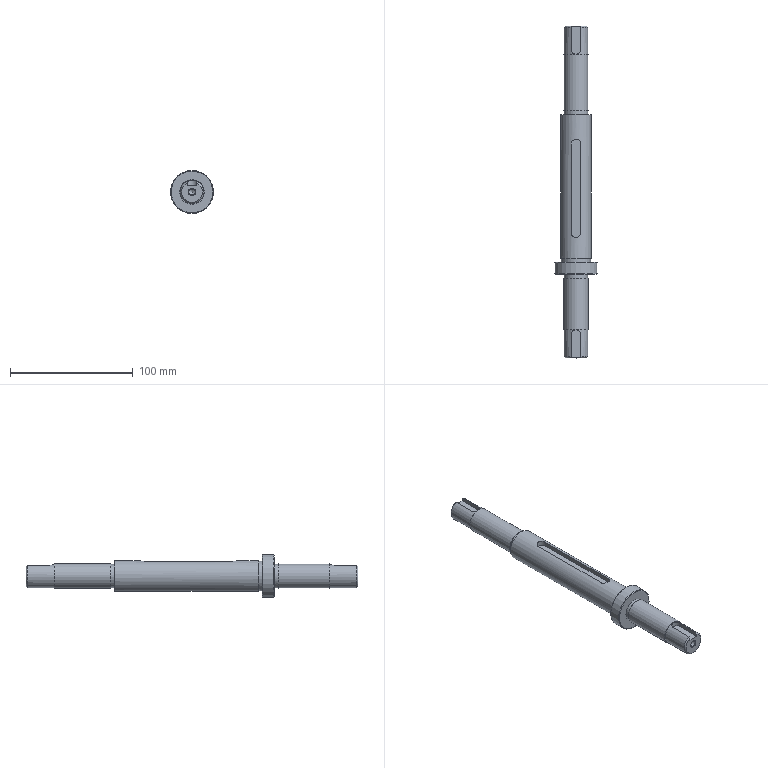Part | STEP file | 冲床-300配套压波_id562_x_t | 1 solid | 49 faces | box 35 x 270 x 35 mm | volume 104906 mm3 | plane 21 | cylinder 17 | cone 11 | commonest cylinder face diameters 19 x4 5 x2 6.8 x2 8 x2 8.04 x2 20 x2
STEP:
#1=CARTESIAN_POINT('',(1267.,-67.,104.));
#2=VERTEX_POINT('',#1);
#3=CARTESIAN_POINT('',(1250.,-67.,104.));
#4=DIRECTION('',(0.,-1.,0.));
#5=DIRECTION('',(1.,0.,0.));
#6=AXIS2_PLACEMENT_3D('',#3,#4,#5);
#7=CIRCLE('',#6,17.);
#8=EDGE_CURVE('',#2,#2,#7,.T.);
#9=ORIENTED_EDGE('',*,*,#8,.T.);
#10=EDGE_LOOP('',(#9));
#11=FACE_BOUND('',#10,.T.);
#12=CARTESIAN_POINT('',(1259.5,-67.,104.));
#13=VERTEX_POINT('',#12);
#14=CARTESIAN_POINT('',(1250.,-67.,104.));
#15=DIRECTION('',(0.,-1.,0.));
#16=DIRECTION('',(1.,0.,0.));
#17=AXIS2_PLACEMENT_3D('',#14,#15,#16);
#18=CIRCLE('',#17,9.5);
#19=EDGE_CURVE('',#13,#13,#18,.T.);
#20=ORIENTED_EDGE('',*,*,#19,.F.);
#21=EDGE_LOOP('',(#20));
#22=FACE_BOUND('',#21,.T.);
#23=CARTESIAN_POINT('',(1250.,-67.,104.));
#24=DIRECTION('',(0.,-1.,0.));
#25=DIRECTION('',(1.,0.,0.));
#26=AXIS2_PLACEMENT_3D('',#23,#24,#25);
#27=PLANE('',#26);
#28=ADVANCED_FACE('',(#11,#22),#27,.T.);
#29=CARTESIAN_POINT('',(1233.,-57.,104.));
#30=VERTEX_POINT('',#29);
#31=CARTESIAN_POINT('',(1250.,-57.,104.));
#32=DIRECTION('',(0.,1.,0.));
#33=DIRECTION('',(-1.,0.,0.));
#34=AXIS2_PLACEMENT_3D('',#31,#32,#33);
#35=CIRCLE('',#34,17.);
#36=EDGE_CURVE('',#30,#30,#35,.T.);
#37=ORIENTED_EDGE('',*,*,#36,.T.);
#38=EDGE_LOOP('',(#37));
#39=FACE_BOUND('',#38,.T.);
#40=CARTESIAN_POINT('',(1238.,-57.,104.));
#41=VERTEX_POINT('',#40);
#42=CARTESIAN_POINT('',(1250.,-57.,104.));
#43=DIRECTION('',(0.,1.,0.));
#44=DIRECTION('',(-1.,0.,0.));
#45=AXIS2_PLACEMENT_3D('',#42,#43,#44);
#46=CIRCLE('',#45,12.);
#47=EDGE_CURVE('',#41,#41,#46,.T.);
#48=ORIENTED_EDGE('',*,*,#47,.F.);
#49=EDGE_LOOP('',(#48));
#50=FACE_BOUND('',#49,.T.);
#51=CARTESIAN_POINT('',(1250.,-57.,104.));
#52=DIRECTION('',(0.,1.,0.));
#53=DIRECTION('',(-1.,0.,0.));
#54=AXIS2_PLACEMENT_3D('',#51,#52,#53);
#55=PLANE('',#54);
#56=ADVANCED_FACE('',(#39,#50),#55,.T.);
#57=CARTESIAN_POINT('',(1250.,-66.5,121.5));
#58=VERTEX_POINT('',#57);
#59=CARTESIAN_POINT('',(1250.,-66.5,104.));
#60=DIRECTION('',(0.,1.,0.));
#61=DIRECTION('',(0.,0.,1.));
#62=AXIS2_PLACEMENT_3D('',#59,#60,#61);
#63=CIRCLE('',#62,17.5);
#64=EDGE_CURVE('',#58,#58,#63,.T.);
#65=ORIENTED_EDGE('',*,*,#64,.T.);
#66=EDGE_LOOP('',(#65));
#67=FACE_BOUND('',#66,.T.);
#68=CARTESIAN_POINT('',(1250.,-57.5,86.5));
#69=VERTEX_POINT('',#68);
#70=CARTESIAN_POINT('',(1250.,-57.5,104.));
#71=DIRECTION('',(0.,-1.,0.));
#72=DIRECTION('',(0.,0.,-1.));
#73=AXIS2_PLACEMENT_3D('',#70,#71,#72);
#74=CIRCLE('',#73,17.5);
#75=EDGE_CURVE('',#69,#69,#74,.T.);
#76=ORIENTED_EDGE('',*,*,#75,.T.);
#77=EDGE_LOOP('',(#76));
#78=FACE_BOUND('',#77,.T.);
#79=CARTESIAN_POINT('',(1250.,-54.,104.));
#80=DIRECTION('',(0.,-1.,0.));
#81=DIRECTION('',(1.,0.,0.));
#82=AXIS2_PLACEMENT_3D('',#79,#80,#81);
#83=CYLINDRICAL_SURFACE('',#82,17.5);
#84=ADVANCED_FACE('',(#67,#78),#83,.T.);
#85=ORIENTED_EDGE('',*,*,#8,.F.);
#86=EDGE_LOOP('',(#85));
#87=FACE_BOUND('',#86,.T.);
#88=ORIENTED_EDGE('',*,*,#64,.F.);
#89=EDGE_LOOP('',(#88));
#90=FACE_BOUND('',#89,.T.);
#91=CARTESIAN_POINT('',(1250.,-66.5,104.));
#92=DIRECTION('',(0.,1.,0.));
#93=DIRECTION('',(0.,0.,1.));
#94=AXIS2_PLACEMENT_3D('',#91,#92,#93);
#95=CONICAL_SURFACE('',#94,17.5,45.);
#96=ADVANCED_FACE('',(#87,#90),#95,.T.);
#97=ORIENTED_EDGE('',*,*,#36,.F.);
#98=EDGE_LOOP('',(#97));
#99=FACE_BOUND('',#98,.T.);
#100=ORIENTED_EDGE('',*,*,#75,.F.);
#101=EDGE_LOOP('',(#100));
#102=FACE_BOUND('',#101,.T.);
#103=CARTESIAN_POINT('',(1250.,-57.5,104.));
#104=DIRECTION('',(0.,-1.,0.));
#105=DIRECTION('',(0.,0.,-1.));
#106=AXIS2_PLACEMENT_3D('',#103,#104,#105);
#107=CONICAL_SURFACE('',#106,17.5,45.);
#108=ADVANCED_FACE('',(#99,#102),#107,.T.);
#109=CARTESIAN_POINT('',(1250.,-54.,92.));
#110=VERTEX_POINT('',#109);
#111=CARTESIAN_POINT('',(1250.,-54.,104.));
#112=DIRECTION('',(0.,-1.,0.));
#113=DIRECTION('',(0.,0.,-1.));
#114=AXIS2_PLACEMENT_3D('',#111,#112,#113);
#115=CIRCLE('',#114,12.);
#116=EDGE_CURVE('',#110,#110,#115,.T.);
#117=ORIENTED_EDGE('',*,*,#116,.F.);
#118=EDGE_LOOP('',(#117));
#119=FACE_BOUND('',#118,.T.);
#120=CARTESIAN_POINT('',(1237.5,-54.,104.));
#121=VERTEX_POINT('',#120);
#122=CARTESIAN_POINT('',(1250.,-54.,104.));
#123=DIRECTION('',(0.,1.,0.));
#124=DIRECTION('',(-1.,0.,0.));
#125=AXIS2_PLACEMENT_3D('',#122,#123,#124);
#126=CIRCLE('',#125,12.5);
#127=EDGE_CURVE('',#121,#121,#126,.T.);
#128=ORIENTED_EDGE('',*,*,#127,.F.);
#129=EDGE_LOOP('',(#128));
#130=FACE_BOUND('',#129,.T.);
#131=CARTESIAN_POINT('',(1250.,-54.,104.));
#132=DIRECTION('',(0.,-1.,0.));
#133=DIRECTION('',(0.,0.,-1.));
#134=AXIS2_PLACEMENT_3D('',#131,#132,#133);
#135=PLANE('',#134);
#136=ADVANCED_FACE('',(#119,#130),#135,.T.);
#137=ORIENTED_EDGE('',*,*,#47,.T.);
#138=EDGE_LOOP('',(#137));
#139=FACE_BOUND('',#138,.T.);
#140=ORIENTED_EDGE('',*,*,#116,.T.);
#141=EDGE_LOOP('',(#140));
#142=FACE_BOUND('',#141,.T.);
#143=CARTESIAN_POINT('',(1250.,-57.,104.));
#144=DIRECTION('',(0.,1.,0.));
#145=DIRECTION('',(0.,0.,1.));
#146=AXIS2_PLACEMENT_3D('',#143,#144,#145);
#147=CYLINDRICAL_SURFACE('',#146,12.);
#148=ADVANCED_FACE('',(#139,#142),#147,.T.);
#149=CARTESIAN_POINT('',(1250.,66.,114.));
#150=VERTEX_POINT('',#149);
#151=CARTESIAN_POINT('',(1250.,66.,104.));
#152=DIRECTION('',(0.,-1.,0.));
#153=DIRECTION('',(0.,0.,1.));
#154=AXIS2_PLACEMENT_3D('',#151,#152,#153);
#155=CIRCLE('',#154,10.);
#156=EDGE_CURVE('',#150,#150,#155,.T.);
#157=ORIENTED_EDGE('',*,*,#156,.F.);
#158=EDGE_LOOP('',(#157));
#159=FACE_BOUND('',#158,.T.);
#160=CARTESIAN_POINT('',(1250.,112.,114.));
#161=VERTEX_POINT('',#160);
#162=CARTESIAN_POINT('',(1250.,112.,104.));
#163=DIRECTION('',(0.,-1.,0.));
#164=DIRECTION('',(0.,0.,1.));
#165=AXIS2_PLACEMENT_3D('',#162,#163,#164);
#166=CIRCLE('',#165,10.);
#167=EDGE_CURVE('',#161,#161,#166,.T.);
#168=ORIENTED_EDGE('',*,*,#167,.T.);
#169=EDGE_LOOP('',(#168));
#170=FACE_BOUND('',#169,.T.);
#171=CARTESIAN_POINT('',(1250.,92.,104.));
#172=DIRECTION('',(0.,1.,0.));
#173=DIRECTION('',(1.,0.,0.));
#174=AXIS2_PLACEMENT_3D('',#171,#172,#173);
#175=CYLINDRICAL_SURFACE('',#174,10.);
#176=ADVANCED_FACE('',(#159,#170),#175,.T.);
#177=ORIENTED_EDGE('',*,*,#156,.T.);
#178=EDGE_LOOP('',(#177));
#179=FACE_BOUND('',#178,.T.);
#180=CARTESIAN_POINT('',(1250.,66.,113.5));
#181=VERTEX_POINT('',#180);
#182=CARTESIAN_POINT('',(1250.,66.,104.));
#183=DIRECTION('',(0.,-1.,0.));
#184=DIRECTION('',(0.,0.,1.));
#185=AXIS2_PLACEMENT_3D('',#182,#183,#184);
#186=CIRCLE('',#185,9.5);
#187=EDGE_CURVE('',#181,#181,#186,.T.);
#188=ORIENTED_EDGE('',*,*,#187,.F.);
#189=EDGE_LOOP('',(#188));
#190=FACE_BOUND('',#189,.T.);
#191=CARTESIAN_POINT('',(1250.,66.,104.));
#192=DIRECTION('',(0.,1.,0.));
#193=DIRECTION('',(0.,0.,1.));
#194=AXIS2_PLACEMENT_3D('',#191,#192,#193);
#195=PLANE('',#194);
#196=ADVANCED_FACE('',(#179,#190),#195,.F.);
#197=CARTESIAN_POINT('',(1250.,63.,94.5));
#198=VERTEX_POINT('',#197);
#199=CARTESIAN_POINT('',(1250.,63.,104.));
#200=DIRECTION('',(0.,1.,0.));
#201=DIRECTION('',(0.,0.,-1.));
#202=AXIS2_PLACEMENT_3D('',#199,#200,#201);
#203=CIRCLE('',#202,9.5);
#204=EDGE_CURVE('',#198,#198,#203,.T.);
#205=ORIENTED_EDGE('',*,*,#204,.T.);
#206=EDGE_LOOP('',(#205));
#207=FACE_BOUND('',#206,.T.);
#208=ORIENTED_EDGE('',*,*,#187,.T.);
#209=EDGE_LOOP('',(#208));
#210=FACE_BOUND('',#209,.T.);
#211=CARTESIAN_POINT('',(1250.,92.,104.));
#212=DIRECTION('',(0.,1.,0.));
#213=DIRECTION('',(0.,0.,1.));
#214=AXIS2_PLACEMENT_3D('',#211,#212,#213);
#215=CYLINDRICAL_SURFACE('',#214,9.5);
#216=ADVANCED_FACE('',(#207,#210),#215,.T.);
#217=CARTESIAN_POINT('',(1254.02,38.98,112.3));
#218=VERTEX_POINT('',#217);
#219=CARTESIAN_POINT('',(1245.98,38.98,112.3));
#220=VERTEX_POINT('',#219);
#221=CARTESIAN_POINT('',(1250.,38.98,112.3));
#222=DIRECTION('',(0.,0.,1.));
#223=DIRECTION('',(1.,0.,0.));
#224=AXIS2_PLACEMENT_3D('',#221,#222,#223);
#225=CIRCLE('',#224,4.02);
#226=EDGE_CURVE('',#218,#220,#225,.T.);
#227=ORIENTED_EDGE('',*,*,#226,.T.);
#228=CARTESIAN_POINT('',(1245.98,-32.98,112.3));
#229=VERTEX_POINT('',#228);
#230=CARTESIAN_POINT('',(1245.98,43.,112.3));
#231=DIRECTION('',(0.,1.,0.));
#232=VECTOR('',#231,1.);
#233=LINE('',#230,#232);
#234=EDGE_CURVE('',#229,#220,#233,.T.);
#235=ORIENTED_EDGE('',*,*,#234,.F.);
#236=CARTESIAN_POINT('',(1254.02,-32.98,112.3));
#237=VERTEX_POINT('',#236);
#238=CARTESIAN_POINT('',(1250.,-32.98,112.3));
#239=DIRECTION('',(0.,0.,1.));
#240=DIRECTION('',(1.,0.,0.));
#241=AXIS2_PLACEMENT_3D('',#238,#239,#240);
#242=CIRCLE('',#241,4.02);
#243=EDGE_CURVE('',#229,#237,#242,.T.);
#244=ORIENTED_EDGE('',*,*,#243,.T.);
#245=CARTESIAN_POINT('',(1254.02,43.,112.3));
#246=DIRECTION('',(0.,1.,0.));
#247=VECTOR('',#246,1.);
#248=LINE('',#245,#247);
#249=EDGE_CURVE('',#237,#218,#248,.T.);
#250=ORIENTED_EDGE('',*,*,#249,.T.);
#251=EDGE_LOOP('',(#227,#235,#244,#250));
#252=FACE_OUTER_BOUND('',#251,.T.);
#253=CARTESIAN_POINT('',(1254.02,43.,112.3));
#254=DIRECTION('',(0.,0.,1.));
#255=DIRECTION('',(1.,0.,0.));
#256=AXIS2_PLACEMENT_3D('',#253,#254,#255);
#257=PLANE('',#256);
#258=ADVANCED_FACE('',(#252),#257,.T.);
#259=CARTESIAN_POINT('',(1250.,63.,91.5));
#260=VERTEX_POINT('',#259);
#261=CARTESIAN_POINT('',(1250.,63.,104.));
#262=DIRECTION('',(0.,1.,0.));
#263=DIRECTION('',(0.,0.,-1.));
#264=AXIS2_PLACEMENT_3D('',#261,#262,#263);
#265=CIRCLE('',#264,12.5);
#266=EDGE_CURVE('',#260,#260,#265,.T.);
#267=ORIENTED_EDGE('',*,*,#266,.T.);
#268=EDGE_LOOP('',(#267));
#269=FACE_BOUND('',#268,.T.);
#270=ORIENTED_EDGE('',*,*,#204,.F.);
#271=EDGE_LOOP('',(#270));
#272=FACE_BOUND('',#271,.T.);
#273=CARTESIAN_POINT('',(1250.,63.,104.));
#274=DIRECTION('',(0.,-1.,0.));
#275=DIRECTION('',(0.,0.,1.));
#276=AXIS2_PLACEMENT_3D('',#273,#274,#275);
#277=PLANE('',#276);
#278=ADVANCED_FACE('',(#269,#272),#277,.F.);
#279=CARTESIAN_POINT('',(1254.02,-32.98,115.836));
#280=VERTEX_POINT('',#279);
#281=CARTESIAN_POINT('',(1254.02,-32.98,116.5));
#282=DIRECTION('',(0.,0.,1.));
#283=VECTOR('',#282,1.);
#284=LINE('',#281,#283);
#285=EDGE_CURVE('',#237,#280,#284,.T.);
#286=ORIENTED_EDGE('',*,*,#285,.F.);
#287=ORIENTED_EDGE('',*,*,#243,.F.);
#288=CARTESIAN_POINT('',(1245.98,-32.98,115.836));
#289=VERTEX_POINT('',#288);
#290=CARTESIAN_POINT('',(1245.98,-32.98,112.4));
#291=DIRECTION('',(0.,0.,-1.));
#292=VECTOR('',#291,1.);
#293=LINE('',#290,#292);
#294=EDGE_CURVE('',#289,#229,#293,.T.);
#295=ORIENTED_EDGE('',*,*,#294,.F.);
#296=CARTESIAN_POINT('',(1254.02,-32.98,115.836));
#297=CARTESIAN_POINT('',(1254.02,-33.417,115.836));
#298=CARTESIAN_POINT('',(1253.947,-33.86,115.862));
#299=CARTESIAN_POINT('',(1253.807,-34.271,115.906));
#300=CARTESIAN_POINT('',(1253.668,-34.682,115.951));
#301=CARTESIAN_POINT('',(1253.459,-35.073,116.015));
#302=CARTESIAN_POINT('',(1253.198,-35.416,116.084));
#303=CARTESIAN_POINT('',(1252.928,-35.77,116.155));
#304=CARTESIAN_POINT('',(1252.596,-36.082,116.233));
#305=CARTESIAN_POINT('',(1252.224,-36.328,116.3));
#306=CARTESIAN_POINT('',(1251.844,-36.581,116.369));
#307=CARTESIAN_POINT('',(1251.413,-36.772,116.428));
#308=CARTESIAN_POINT('',(1250.966,-36.882,116.463));
#309=CARTESIAN_POINT('',(1250.535,-36.989,116.496));
#310=CARTESIAN_POINT('',(1250.076,-37.024,116.508));
#311=CARTESIAN_POINT('',(1249.632,-36.983,116.495));
#312=CARTESIAN_POINT('',(1249.204,-36.944,116.482));
#313=CARTESIAN_POINT('',(1248.778,-36.833,116.446));
#314=CARTESIAN_POINT('',(1248.387,-36.662,116.395));
#315=CARTESIAN_POINT('',(1247.99,-36.488,116.344));
#316=CARTESIAN_POINT('',(1247.62,-36.248,116.276));
#317=CARTESIAN_POINT('',(1247.301,-35.959,116.205));
#318=CARTESIAN_POINT('',(1246.969,-35.658,116.132));
#319=CARTESIAN_POINT('',(1246.683,-35.296,116.054));
#320=CARTESIAN_POINT('',(1246.468,-34.9,115.991));
#321=CARTESIAN_POINT('',(1246.251,-34.5,115.927));
#322=CARTESIAN_POINT('',(1246.099,-34.053,115.876));
#323=CARTESIAN_POINT('',(1246.028,-33.599,115.852));
#324=CARTESIAN_POINT('',(1245.996,-33.395,115.841));
#325=CARTESIAN_POINT('',(1245.98,-33.187,115.836));
#326=CARTESIAN_POINT('',(1245.98,-32.98,115.836));
#327=B_SPLINE_CURVE_WITH_KNOTS('',3,(#296,#297,#298,#299,#300,#301,#302,#303,#304,#305,#306,#307,#308,#309,#310,#311,#312,#313,#314,#315,#316,#317,#318,#319,#320,#321,#322,#323,#324,#325,#326),.UNSPECIFIED.,.F.,.F.,(4,3,3,3,3,3,3,3,3,3,4),(0.,0.1036,0.207,0.3138,0.4233,0.5292,0.6311,0.7343,0.8422,0.9514,1.),.UNSPECIFIED.);
#328=EDGE_CURVE('',#280,#289,#327,.T.);
#329=ORIENTED_EDGE('',*,*,#328,.F.);
#330=EDGE_LOOP('',(#286,#287,#295,#329));
#331=FACE_OUTER_BOUND('',#330,.T.);
#332=CARTESIAN_POINT('',(1250.,-32.98,116.5));
#333=DIRECTION('',(0.,0.,-1.));
#334=DIRECTION('',(-1.,0.,0.));
#335=AXIS2_PLACEMENT_3D('',#332,#333,#334);
#336=CYLINDRICAL_SURFACE('',#335,4.02);
#337=ADVANCED_FACE('',(#331),#336,.F.);
#338=CARTESIAN_POINT('',(1254.02,38.98,115.836));
#339=VERTEX_POINT('',#338);
#340=CARTESIAN_POINT('',(1254.02,173.,115.836));
#341=DIRECTION('',(0.,1.,0.));
#342=VECTOR('',#341,1.);
#343=LINE('',#340,#342);
#344=EDGE_CURVE('',#280,#339,#343,.T.);
#345=ORIENTED_EDGE('',*,*,#344,.T.);
#346=CARTESIAN_POINT('',(1254.02,38.98,116.5));
#347=DIRECTION('',(0.,0.,-1.));
#348=VECTOR('',#347,1.);
#349=LINE('',#346,#348);
#350=EDGE_CURVE('',#339,#218,#349,.T.);
#351=ORIENTED_EDGE('',*,*,#350,.T.);
#352=ORIENTED_EDGE('',*,*,#249,.F.);
#353=ORIENTED_EDGE('',*,*,#285,.T.);
#354=EDGE_LOOP('',(#345,#351,#352,#353));
#355=FACE_OUTER_BOUND('',#354,.T.);
#356=CARTESIAN_POINT('',(1254.02,43.,116.5));
#357=DIRECTION('',(-1.,0.,0.));
#358=DIRECTION('',(0.,0.,1.));
#359=AXIS2_PLACEMENT_3D('',#356,#357,#358);
#360=PLANE('',#359);
#361=ADVANCED_FACE('',(#355),#360,.T.);
#362=CARTESIAN_POINT('',(1245.98,38.98,115.836));
#363=VERTEX_POINT('',#362);
#364=CARTESIAN_POINT('',(1245.98,38.98,112.4));
#365=DIRECTION('',(0.,0.,1.));
#366=VECTOR('',#365,1.);
#367=LINE('',#364,#366);
#368=EDGE_CURVE('',#220,#363,#367,.T.);
#369=ORIENTED_EDGE('',*,*,#368,.F.);
#370=ORIENTED_EDGE('',*,*,#226,.F.);
#371=ORIENTED_EDGE('',*,*,#350,.F.);
#372=CARTESIAN_POINT('',(1245.98,38.98,115.836));
#373=CARTESIAN_POINT('',(1245.98,39.417,115.836));
#374=CARTESIAN_POINT('',(1246.053,39.86,115.862));
#375=CARTESIAN_POINT('',(1246.193,40.271,115.906));
#376=CARTESIAN_POINT('',(1246.332,40.682,115.951));
#377=CARTESIAN_POINT('',(1246.541,41.073,116.015));
#378=CARTESIAN_POINT('',(1246.802,41.416,116.084));
#379=CARTESIAN_POINT('',(1247.072,41.77,116.155));
#380=CARTESIAN_POINT('',(1247.404,42.082,116.233));
#381=CARTESIAN_POINT('',(1247.776,42.328,116.3));
#382=CARTESIAN_POINT('',(1248.156,42.581,116.369));
#383=CARTESIAN_POINT('',(1248.587,42.772,116.428));
#384=CARTESIAN_POINT('',(1249.034,42.882,116.463));
#385=CARTESIAN_POINT('',(1249.465,42.989,116.496));
#386=CARTESIAN_POINT('',(1249.924,43.024,116.508));
#387=CARTESIAN_POINT('',(1250.368,42.983,116.495));
#388=CARTESIAN_POINT('',(1250.796,42.944,116.482));
#389=CARTESIAN_POINT('',(1251.222,42.833,116.446));
#390=CARTESIAN_POINT('',(1251.613,42.662,116.395));
#391=CARTESIAN_POINT('',(1252.01,42.488,116.344));
#392=CARTESIAN_POINT('',(1252.38,42.248,116.276));
#393=CARTESIAN_POINT('',(1252.699,41.959,116.205));
#394=CARTESIAN_POINT('',(1253.031,41.658,116.132));
#395=CARTESIAN_POINT('',(1253.317,41.296,116.054));
#396=CARTESIAN_POINT('',(1253.532,40.9,115.991));
#397=CARTESIAN_POINT('',(1253.749,40.5,115.927));
#398=CARTESIAN_POINT('',(1253.901,40.053,115.876));
#399=CARTESIAN_POINT('',(1253.972,39.599,115.852));
#400=CARTESIAN_POINT('',(1254.004,39.395,115.841));
#401=CARTESIAN_POINT('',(1254.02,39.187,115.836));
#402=CARTESIAN_POINT('',(1254.02,38.98,115.836));
#403=B_SPLINE_CURVE_WITH_KNOTS('',3,(#372,#373,#374,#375,#376,#377,#378,#379,#380,#381,#382,#383,#384,#385,#386,#387,#388,#389,#390,#391,#392,#393,#394,#395,#396,#397,#398,#399,#400,#401,#402),.UNSPECIFIED.,.F.,.F.,(4,3,3,3,3,3,3,3,3,3,4),(0.,0.1036,0.207,0.3138,0.4233,0.5292,0.6311,0.7343,0.8422,0.9514,1.),.UNSPECIFIED.);
#404=EDGE_CURVE('',#363,#339,#403,.T.);
#405=ORIENTED_EDGE('',*,*,#404,.F.);
#406=EDGE_LOOP('',(#369,#370,#371,#405));
#407=FACE_OUTER_BOUND('',#406,.T.);
#408=CARTESIAN_POINT('',(1250.,38.98,0.));
#409=DIRECTION('',(0.,0.,-1.));
#410=DIRECTION('',(-1.,0.,0.));
#411=AXIS2_PLACEMENT_3D('',#408,#409,#410);
#412=CYLINDRICAL_SURFACE('',#411,4.02);
#413=ADVANCED_FACE('',(#407),#412,.F.);
#414=CARTESIAN_POINT('',(1245.98,173.,115.836));
#415=DIRECTION('',(0.,-1.,0.));
#416=VECTOR('',#415,1.);
#417=LINE('',#414,#416);
#418=EDGE_CURVE('',#363,#289,#417,.T.);
#419=ORIENTED_EDGE('',*,*,#418,.T.);
#420=ORIENTED_EDGE('',*,*,#294,.T.);
#421=ORIENTED_EDGE('',*,*,#234,.T.);
#422=ORIENTED_EDGE('',*,*,#368,.T.);
#423=EDGE_LOOP('',(#419,#420,#421,#422));
#424=FACE_OUTER_BOUND('',#423,.T.);
#425=CARTESIAN_POINT('',(1245.98,43.,112.4));
#426=DIRECTION('',(1.,0.,0.));
#427=DIRECTION('',(0.,0.,-1.));
#428=AXIS2_PLACEMENT_3D('',#425,#426,#427);
#429=PLANE('',#428);
#430=ADVANCED_FACE('',(#424),#429,.T.);
#431=ORIENTED_EDGE('',*,*,#127,.T.);
#432=EDGE_LOOP('',(#431));
#433=FACE_BOUND('',#432,.T.);
#434=ORIENTED_EDGE('',*,*,#418,.F.);
#435=ORIENTED_EDGE('',*,*,#404,.T.);
#436=ORIENTED_EDGE('',*,*,#344,.F.);
#437=ORIENTED_EDGE('',*,*,#328,.T.);
#438=EDGE_LOOP('',(#434,#435,#436,#437));
#439=FACE_BOUND('',#438,.T.);
#440=ORIENTED_EDGE('',*,*,#266,.F.);
#441=EDGE_LOOP('',(#440));
#442=FACE_BOUND('',#441,.T.);
#443=CARTESIAN_POINT('',(1250.,181.,104.));
#444=DIRECTION('',(0.,-1.,0.));
#445=DIRECTION('',(0.,0.,-1.));
#446=AXIS2_PLACEMENT_3D('',#443,#444,#445);
#447=CYLINDRICAL_SURFACE('',#446,12.5);
#448=ADVANCED_FACE('',(#433,#439,#442),#447,.T.);
#449=CARTESIAN_POINT('',(1250.,-70.,113.5));
#450=VERTEX_POINT('',#449);
#451=CARTESIAN_POINT('',(1250.,-70.,104.));
#452=DIRECTION('',(0.,1.,0.));
#453=DIRECTION('',(0.,0.,1.));
#454=AXIS2_PLACEMENT_3D('',#451,#452,#453);
#455=CIRCLE('',#454,9.5);
#456=EDGE_CURVE('',#450,#450,#455,.T.);
#457=ORIENTED_EDGE('',*,*,#456,.F.);
#458=EDGE_LOOP('',(#457));
#459=FACE_BOUND('',#458,.T.);
#460=CARTESIAN_POINT('',(1260.,-70.,104.));
#461=VERTEX_POINT('',#460);
#462=CARTESIAN_POINT('',(1250.,-70.,104.));
#463=DIRECTION('',(0.,-1.,0.));
#464=DIRECTION('',(1.,0.,0.));
#465=AXIS2_PLACEMENT_3D('',#462,#463,#464);
#466=CIRCLE('',#465,10.);
#467=EDGE_CURVE('',#461,#461,#466,.T.);
#468=ORIENTED_EDGE('',*,*,#467,.F.);
#469=EDGE_LOOP('',(#468));
#470=FACE_BOUND('',#469,.T.);
#471=CARTESIAN_POINT('',(1250.,-70.,104.));
#472=DIRECTION('',(0.,1.,0.));
#473=DIRECTION('',(0.,0.,1.));
#474=AXIS2_PLACEMENT_3D('',#471,#472,#473);
#475=PLANE('',#474);
#476=ADVANCED_FACE('',(#459,#470),#475,.T.);
#477=ORIENTED_EDGE('',*,*,#19,.T.);
#478=EDGE_LOOP('',(#477));
#479=FACE_BOUND('',#478,.T.);
#480=ORIENTED_EDGE('',*,*,#456,.T.);
#481=EDGE_LOOP('',(#480));
#482=FACE_BOUND('',#481,.T.);
#483=CARTESIAN_POINT('',(1250.,-67.,104.));
#484=DIRECTION('',(0.,-1.,0.));
#485=DIRECTION('',(0.,0.,-1.));
#486=AXIS2_PLACEMENT_3D('',#483,#484,#485);
#487=CYLINDRICAL_SURFACE('',#486,9.5);
#488=ADVANCED_FACE('',(#479,#482),#487,.T.);
#489=ORIENTED_EDGE('',*,*,#467,.T.);
#490=EDGE_LOOP('',(#489));
#491=FACE_BOUND('',#490,.T.);
#492=CARTESIAN_POINT('',(1260.,-112.,104.));
#493=VERTEX_POINT('',#492);
#494=CARTESIAN_POINT('',(1250.,-112.,104.));
#495=DIRECTION('',(0.,-1.,0.));
#496=DIRECTION('',(1.,0.,0.));
#497=AXIS2_PLACEMENT_3D('',#494,#495,#496);
#498=CIRCLE('',#497,10.);
#499=EDGE_CURVE('',#493,#493,#498,.T.);
#500=ORIENTED_EDGE('',*,*,#499,.F.);
#501=EDGE_LOOP('',(#500));
#502=FACE_BOUND('',#501,.T.);
#503=CARTESIAN_POINT('',(1250.,-70.,104.));
#504=DIRECTION('',(0.,-1.,0.));
#505=DIRECTION('',(1.,0.,0.));
#506=AXIS2_PLACEMENT_3D('',#503,#504,#505);
#507=CYLINDRICAL_SURFACE('',#506,10.);
#508=ADVANCED_FACE('',(#491,#502),#507,.T.);
#509=CARTESIAN_POINT('',(1250.,-115.,106.5));
#510=VERTEX_POINT('',#509);
#511=CARTESIAN_POINT('',(1250.,-115.,104.));
#512=DIRECTION('',(0.,-1.,0.));
#513=DIRECTION('',(0.,0.,1.));
#514=AXIS2_PLACEMENT_3D('',#511,#512,#513);
#515=CIRCLE('',#514,2.5);
#516=EDGE_CURVE('',#510,#510,#515,.T.);
#517=ORIENTED_EDGE('',*,*,#516,.T.);
#518=EDGE_LOOP('',(#517));
#519=FACE_BOUND('',#518,.T.);
#520=CARTESIAN_POINT('',(1250.,-113.498,104.));
#521=VERTEX_POINT('',#520);
#522=VERTEX_LOOP('',#521);
#523=FACE_BOUND('',#522,.T.);
#524=CARTESIAN_POINT('',(1250.,-115.,104.));
#525=DIRECTION('',(0.,-1.,0.));
#526=DIRECTION('',(0.,0.,-1.));
#527=AXIS2_PLACEMENT_3D('',#524,#525,#526);
#528=CONICAL_SURFACE('',#527,2.5,59.);
#529=ADVANCED_FACE('',(#519,#523),#528,.F.);
#530=CARTESIAN_POINT('',(1250.,-134.5,101.5));
#531=VERTEX_POINT('',#530);
#532=CARTESIAN_POINT('',(1250.,-134.5,104.));
#533=DIRECTION('',(0.,-1.,0.));
#534=DIRECTION('',(0.,0.,-1.));
#535=AXIS2_PLACEMENT_3D('',#532,#533,#534);
#536=CIRCLE('',#535,2.5);
#537=EDGE_CURVE('',#531,#531,#536,.T.);
#538=ORIENTED_EDGE('',*,*,#537,.T.);
#539=EDGE_LOOP('',(#538));
#540=FACE_BOUND('',#539,.T.);
#541=ORIENTED_EDGE('',*,*,#516,.F.);
#542=EDGE_LOOP('',(#541));
#543=FACE_BOUND('',#542,.T.);
#544=CARTESIAN_POINT('',(1250.,-135.,104.));
#545=DIRECTION('',(0.,1.,0.));
#546=DIRECTION('',(0.,0.,1.));
#547=AXIS2_PLACEMENT_3D('',#544,#545,#546);
#548=CYLINDRICAL_SURFACE('',#547,2.5);
#549=ADVANCED_FACE('',(#540,#543),#548,.F.);
#550=ORIENTED_EDGE('',*,*,#537,.F.);
#551=EDGE_LOOP('',(#550));
#552=FACE_BOUND('',#551,.T.);
#553=CARTESIAN_POINT('',(1250.,-135.,101.));
#554=VERTEX_POINT('',#553);
#555=CARTESIAN_POINT('',(1250.,-135.,104.));
#556=DIRECTION('',(0.,1.,0.));
#557=DIRECTION('',(0.,0.,-1.));
#558=AXIS2_PLACEMENT_3D('',#555,#556,#557);
#559=CIRCLE('',#558,3.);
#560=EDGE_CURVE('',#554,#554,#559,.T.);
#561=ORIENTED_EDGE('',*,*,#560,.F.);
#562=EDGE_LOOP('',(#561));
#563=FACE_BOUND('',#562,.T.);
#564=CARTESIAN_POINT('',(1250.,-135.,104.));
#565=DIRECTION('',(0.,-1.,0.));
#566=DIRECTION('',(0.,0.,-1.));
#567=AXIS2_PLACEMENT_3D('',#564,#565,#566);
#568=CONICAL_SURFACE('',#567,3.,45.);
#569=ADVANCED_FACE('',(#552,#563),#568,.F.);
#570=CARTESIAN_POINT('',(1254.,-135.,109.5));
#571=VERTEX_POINT('',#570);
#572=CARTESIAN_POINT('',(1254.,-116.,109.5));
#573=VERTEX_POINT('',#572);
#574=CARTESIAN_POINT('',(1254.,-114.5,109.5));
#575=DIRECTION('',(0.,1.,0.));
#576=VECTOR('',#575,1.);
#577=LINE('',#574,#576);
#578=EDGE_CURVE('',#571,#573,#577,.T.);
#579=ORIENTED_EDGE('',*,*,#578,.T.);
#580=CARTESIAN_POINT('',(1246.,-116.,109.5));
#581=VERTEX_POINT('',#580);
#582=CARTESIAN_POINT('',(1250.,-116.,109.5));
#583=DIRECTION('',(0.,0.,1.));
#584=DIRECTION('',(1.,0.,0.));
#585=AXIS2_PLACEMENT_3D('',#582,#583,#584);
#586=CIRCLE('',#585,4.);
#587=EDGE_CURVE('',#573,#581,#586,.T.);
#588=ORIENTED_EDGE('',*,*,#587,.T.);
#589=CARTESIAN_POINT('',(1246.,-135.,109.5));
#590=VERTEX_POINT('',#589);
#591=CARTESIAN_POINT('',(1246.,-139.499,109.5));
#592=DIRECTION('',(0.,-1.,0.));
#593=VECTOR('',#592,1.);
#594=LINE('',#591,#593);
#595=EDGE_CURVE('',#581,#590,#594,.T.);
#596=ORIENTED_EDGE('',*,*,#595,.T.);
#597=CARTESIAN_POINT('',(1250.,-135.,109.5));
#598=DIRECTION('',(1.,0.,0.));
#599=VECTOR('',#598,1.);
#600=LINE('',#597,#599);
#601=EDGE_CURVE('',#590,#571,#600,.T.);
#602=ORIENTED_EDGE('',*,*,#601,.T.);
#603=EDGE_LOOP('',(#579,#588,#596,#602));
#604=FACE_OUTER_BOUND('',#603,.T.);
#605=CARTESIAN_POINT('',(1250.,-114.5,109.5));
#606=DIRECTION('',(0.,0.,-1.));
#607=DIRECTION('',(-1.,0.,0.));
#608=AXIS2_PLACEMENT_3D('',#605,#606,#607);
#609=PLANE('',#608);
#610=ADVANCED_FACE('',(#604),#609,.F.);
#611=ORIENTED_EDGE('',*,*,#560,.T.);
#612=EDGE_LOOP('',(#611));
#613=FACE_BOUND('',#612,.T.);
#614=CARTESIAN_POINT('',(1246.,-135.,111.5));
#615=VERTEX_POINT('',#614);
#616=CARTESIAN_POINT('',(1246.,-135.,104.));
#617=DIRECTION('',(0.,0.,1.));
#618=VECTOR('',#617,1.);
#619=LINE('',#616,#618);
#620=EDGE_CURVE('',#590,#615,#619,.T.);
#621=ORIENTED_EDGE('',*,*,#620,.T.);
#622=CARTESIAN_POINT('',(1254.,-135.,111.5));
#623=VERTEX_POINT('',#622);
#624=CARTESIAN_POINT('',(1250.,-135.,104.));
#625=DIRECTION('',(0.,-1.,0.));
#626=DIRECTION('',(0.,0.,-1.));
#627=AXIS2_PLACEMENT_3D('',#624,#625,#626);
#628=CIRCLE('',#627,8.5);
#629=EDGE_CURVE('',#615,#623,#628,.T.);
#630=ORIENTED_EDGE('',*,*,#629,.T.);
#631=CARTESIAN_POINT('',(1254.,-135.,104.));
#632=DIRECTION('',(0.,0.,-1.));
#633=VECTOR('',#632,1.);
#634=LINE('',#631,#633);
#635=EDGE_CURVE('',#623,#571,#634,.T.);
#636=ORIENTED_EDGE('',*,*,#635,.T.);
#637=ORIENTED_EDGE('',*,*,#601,.F.);
#638=EDGE_LOOP('',(#621,#630,#636,#637));
#639=FACE_BOUND('',#638,.T.);
#640=CARTESIAN_POINT('',(1250.,-135.,104.));
#641=DIRECTION('',(0.,-1.,0.));
#642=DIRECTION('',(0.,0.,-1.));
#643=AXIS2_PLACEMENT_3D('',#640,#641,#642);
#644=PLANE('',#643);
#645=ADVANCED_FACE('',(#613,#639),#644,.T.);
#646=CARTESIAN_POINT('',(1246.,-116.,112.617));
#647=VERTEX_POINT('',#646);
#648=CARTESIAN_POINT('',(1250.,-112.,113.5));
#649=VERTEX_POINT('',#648);
#650=CARTESIAN_POINT('',(1246.,-116.,112.617));
#651=CARTESIAN_POINT('',(1246.,-114.929,112.617));
#652=CARTESIAN_POINT('',(1246.443,-113.9,112.842));
#653=CARTESIAN_POINT('',(1247.902,-112.442,113.297));
#654=CARTESIAN_POINT('',(1248.941,-112.,113.5));
#655=CARTESIAN_POINT('',(1250.,-112.,113.5));
#656=B_SPLINE_CURVE_WITH_KNOTS('',3,(#650,#651,#652,#653,#654,#655),.UNSPECIFIED.,.F.,.F.,(4,2,4),(0.,0.5,1.),.UNSPECIFIED.);
#657=EDGE_CURVE('',#647,#649,#656,.T.);
#658=ORIENTED_EDGE('',*,*,#657,.F.);
#659=CARTESIAN_POINT('',(1246.,-116.,109.5));
#660=DIRECTION('',(0.,0.,-1.));
#661=VECTOR('',#660,1.);
#662=LINE('',#659,#661);
#663=EDGE_CURVE('',#647,#581,#662,.T.);
#664=ORIENTED_EDGE('',*,*,#663,.T.);
#665=ORIENTED_EDGE('',*,*,#587,.F.);
#666=CARTESIAN_POINT('',(1254.,-116.,112.617));
#667=VERTEX_POINT('',#666);
#668=CARTESIAN_POINT('',(1254.,-116.,109.5));
#669=DIRECTION('',(0.,0.,-1.));
#670=VECTOR('',#669,1.);
#671=LINE('',#668,#670);
#672=EDGE_CURVE('',#667,#573,#671,.T.);
#673=ORIENTED_EDGE('',*,*,#672,.F.);
#674=CARTESIAN_POINT('',(1250.,-112.,113.5));
#675=CARTESIAN_POINT('',(1251.057,-112.,113.5));
#676=CARTESIAN_POINT('',(1252.101,-112.443,113.296));
#677=CARTESIAN_POINT('',(1253.56,-113.904,112.841));
#678=CARTESIAN_POINT('',(1254.,-114.93,112.617));
#679=CARTESIAN_POINT('',(1254.,-116.,112.617));
#680=B_SPLINE_CURVE_WITH_KNOTS('',3,(#674,#675,#676,#677,#678,#679),.UNSPECIFIED.,.F.,.F.,(4,2,4),(0.,0.5,1.),.UNSPECIFIED.);
#681=EDGE_CURVE('',#649,#667,#680,.T.);
#682=ORIENTED_EDGE('',*,*,#681,.F.);
#683=EDGE_LOOP('',(#658,#664,#665,#673,#682));
#684=FACE_OUTER_BOUND('',#683,.T.);
#685=CARTESIAN_POINT('',(1250.,-116.,109.5));
#686=DIRECTION('',(0.,0.,1.));
#687=DIRECTION('',(1.,0.,0.));
#688=AXIS2_PLACEMENT_3D('',#685,#686,#687);
#689=CYLINDRICAL_SURFACE('',#688,4.);
#690=ADVANCED_FACE('',(#684),#689,.F.);
#691=CARTESIAN_POINT('',(1246.,-134.,112.617));
#692=VERTEX_POINT('',#691);
#693=CARTESIAN_POINT('',(1246.,-49.5,112.617));
#694=DIRECTION('',(0.,1.,0.));
#695=VECTOR('',#694,1.);
#696=LINE('',#693,#695);
#697=EDGE_CURVE('',#692,#647,#696,.T.);
#698=ORIENTED_EDGE('',*,*,#697,.F.);
#699=CARTESIAN_POINT('',(1246.,-134.,112.617));
#700=CARTESIAN_POINT('',(1246.,-134.336,112.247));
#701=CARTESIAN_POINT('',(1246.,-134.669,111.875));
#702=CARTESIAN_POINT('',(1246.,-135.,111.5));
#703=B_SPLINE_CURVE_WITH_KNOTS('',3,(#699,#700,#701,#702),.UNSPECIFIED.,.F.,.F.,(4,4),(0.,1.),.UNSPECIFIED.);
#704=EDGE_CURVE('',#692,#615,#703,.T.);
#705=ORIENTED_EDGE('',*,*,#704,.T.);
#706=ORIENTED_EDGE('',*,*,#620,.F.);
#707=ORIENTED_EDGE('',*,*,#595,.F.);
#708=ORIENTED_EDGE('',*,*,#663,.F.);
#709=EDGE_LOOP('',(#698,#705,#706,#707,#708));
#710=FACE_OUTER_BOUND('',#709,.T.);
#711=CARTESIAN_POINT('',(1246.,-139.499,109.5));
#712=DIRECTION('',(1.,0.,0.));
#713=DIRECTION('',(0.,0.,-1.));
#714=AXIS2_PLACEMENT_3D('',#711,#712,#713);
#715=PLANE('',#714);
#716=ADVANCED_FACE('',(#710),#715,.T.);
#717=ORIENTED_EDGE('',*,*,#704,.F.);
#718=CARTESIAN_POINT('',(1254.,-134.,112.617));
#719=VERTEX_POINT('',#718);
#720=CARTESIAN_POINT('',(1250.,-134.,104.));
#721=DIRECTION('',(0.,1.,0.));
#722=DIRECTION('',(0.,0.,-1.));
#723=AXIS2_PLACEMENT_3D('',#720,#721,#722);
#724=CIRCLE('',#723,9.5);
#725=EDGE_CURVE('',#719,#692,#724,.T.);
#726=ORIENTED_EDGE('',*,*,#725,.F.);
#727=CARTESIAN_POINT('',(1254.,-135.,111.5));
#728=CARTESIAN_POINT('',(1254.,-134.669,111.875));
#729=CARTESIAN_POINT('',(1254.,-134.336,112.247));
#730=CARTESIAN_POINT('',(1254.,-134.,112.617));
#731=B_SPLINE_CURVE_WITH_KNOTS('',3,(#727,#728,#729,#730),.UNSPECIFIED.,.F.,.F.,(4,4),(0.,1.),.UNSPECIFIED.);
#732=EDGE_CURVE('',#623,#719,#731,.T.);
#733=ORIENTED_EDGE('',*,*,#732,.F.);
#734=ORIENTED_EDGE('',*,*,#629,.F.);
#735=EDGE_LOOP('',(#717,#726,#733,#734));
#736=FACE_OUTER_BOUND('',#735,.T.);
#737=CARTESIAN_POINT('',(1250.,-135.,104.));
#738=DIRECTION('',(0.,1.,0.));
#739=DIRECTION('',(0.,0.,1.));
#740=AXIS2_PLACEMENT_3D('',#737,#738,#739);
#741=CONICAL_SURFACE('',#740,8.5,45.);
#742=ADVANCED_FACE('',(#736),#741,.T.);
#743=ORIENTED_EDGE('',*,*,#635,.F.);
#744=ORIENTED_EDGE('',*,*,#732,.T.);
#745=CARTESIAN_POINT('',(1254.,-49.5,112.617));
#746=DIRECTION('',(0.,-1.,0.));
#747=VECTOR('',#746,1.);
#748=LINE('',#745,#747);
#749=EDGE_CURVE('',#667,#719,#748,.T.);
#750=ORIENTED_EDGE('',*,*,#749,.F.);
#751=ORIENTED_EDGE('',*,*,#672,.T.);
#752=ORIENTED_EDGE('',*,*,#578,.F.);
#753=EDGE_LOOP('',(#743,#744,#750,#751,#752));
#754=FACE_OUTER_BOUND('',#753,.T.);
#755=CARTESIAN_POINT('',(1254.,-114.5,109.5));
#756=DIRECTION('',(-1.,0.,0.));
#757=DIRECTION('',(0.,-1.,0.));
#758=AXIS2_PLACEMENT_3D('',#755,#756,#757);
#759=PLANE('',#758);
#760=ADVANCED_FACE('',(#754),#759,.T.);
#761=ORIENTED_EDGE('',*,*,#749,.T.);
#762=ORIENTED_EDGE('',*,*,#725,.T.);
#763=ORIENTED_EDGE('',*,*,#697,.T.);
#764=ORIENTED_EDGE('',*,*,#657,.T.);
#765=CARTESIAN_POINT('',(1250.,-112.,104.));
#766=DIRECTION('',(0.,-1.,0.));
#767=DIRECTION('',(1.,0.,0.));
#768=AXIS2_PLACEMENT_3D('',#765,#766,#767);
#769=CIRCLE('',#768,9.5);
#770=EDGE_CURVE('',#649,#649,#769,.T.);
#771=ORIENTED_EDGE('',*,*,#770,.T.);
#772=ORIENTED_EDGE('',*,*,#681,.T.);
#773=EDGE_LOOP('',(#761,#762,#763,#764,#771,#772));
#774=FACE_OUTER_BOUND('',#773,.T.);
#775=CARTESIAN_POINT('',(1250.,-140.,104.));
#776=DIRECTION('',(0.,1.,0.));
#777=DIRECTION('',(-1.,0.,0.));
#778=AXIS2_PLACEMENT_3D('',#775,#776,#777);
#779=CYLINDRICAL_SURFACE('',#778,9.5);
#780=ADVANCED_FACE('',(#774),#779,.T.);
#781=ORIENTED_EDGE('',*,*,#499,.T.);
#782=EDGE_LOOP('',(#781));
#783=FACE_BOUND('',#782,.T.);
#784=ORIENTED_EDGE('',*,*,#770,.F.);
#785=EDGE_LOOP('',(#784));
#786=FACE_BOUND('',#785,.T.);
#787=CARTESIAN_POINT('',(1190.,-112.,183.3));
#788=DIRECTION('',(0.,-1.,0.));
#789=DIRECTION('',(1.,0.,0.));
#790=AXIS2_PLACEMENT_3D('',#787,#788,#789);
#791=PLANE('',#790);
#792=ADVANCED_FACE('',(#783,#786),#791,.T.);
#793=CARTESIAN_POINT('',(1250.,112.,113.5));
#794=VERTEX_POINT('',#793);
#795=CARTESIAN_POINT('',(1250.,112.,104.));
#796=DIRECTION('',(0.,1.,0.));
#797=DIRECTION('',(0.,0.,1.));
#798=AXIS2_PLACEMENT_3D('',#795,#796,#797);
#799=CIRCLE('',#798,9.5);
#800=EDGE_CURVE('',#794,#794,#799,.T.);
#801=ORIENTED_EDGE('',*,*,#800,.F.);
#802=EDGE_LOOP('',(#801));
#803=FACE_BOUND('',#802,.T.);
#804=ORIENTED_EDGE('',*,*,#167,.F.);
#805=EDGE_LOOP('',(#804));
#806=FACE_BOUND('',#805,.T.);
#807=CARTESIAN_POINT('',(1250.,112.,104.));
#808=DIRECTION('',(0.,1.,0.));
#809=DIRECTION('',(0.,0.,1.));
#810=AXIS2_PLACEMENT_3D('',#807,#808,#809);
#811=PLANE('',#810);
#812=ADVANCED_FACE('',(#803,#806),#811,.T.);
#813=CARTESIAN_POINT('',(1246.,134.,112.617));
#814=VERTEX_POINT('',#813);
#815=CARTESIAN_POINT('',(1246.,116.,112.617));
#816=VERTEX_POINT('',#815);
#817=CARTESIAN_POINT('',(1246.,49.5,112.617));
#818=DIRECTION('',(0.,-1.,0.));
#819=VECTOR('',#818,1.);
#820=LINE('',#817,#819);
#821=EDGE_CURVE('',#814,#816,#820,.T.);
#822=ORIENTED_EDGE('',*,*,#821,.F.);
#823=CARTESIAN_POINT('',(1254.,134.,112.617));
#824=VERTEX_POINT('',#823);
#825=CARTESIAN_POINT('',(1250.,134.,104.));
#826=DIRECTION('',(0.,-1.,0.));
#827=DIRECTION('',(0.,0.,1.));
#828=AXIS2_PLACEMENT_3D('',#825,#826,#827);
#829=CIRCLE('',#828,9.5);
#830=EDGE_CURVE('',#814,#824,#829,.T.);
#831=ORIENTED_EDGE('',*,*,#830,.T.);
#832=CARTESIAN_POINT('',(1254.,116.,112.617));
#833=VERTEX_POINT('',#832);
#834=CARTESIAN_POINT('',(1254.,49.5,112.617));
#835=DIRECTION('',(0.,1.,0.));
#836=VECTOR('',#835,1.);
#837=LINE('',#834,#836);
#838=EDGE_CURVE('',#833,#824,#837,.T.);
#839=ORIENTED_EDGE('',*,*,#838,.F.);
#840=CARTESIAN_POINT('',(1250.,112.,113.5));
#841=CARTESIAN_POINT('',(1251.057,112.,113.5));
#842=CARTESIAN_POINT('',(1252.101,112.443,113.296));
#843=CARTESIAN_POINT('',(1253.56,113.904,112.841));
#844=CARTESIAN_POINT('',(1254.,114.93,112.617));
#845=CARTESIAN_POINT('',(1254.,116.,112.617));
#846=B_SPLINE_CURVE_WITH_KNOTS('',3,(#840,#841,#842,#843,#844,#845),.UNSPECIFIED.,.F.,.F.,(4,2,4),(0.,0.5,1.),.UNSPECIFIED.);
#847=EDGE_CURVE('',#794,#833,#846,.T.);
#848=ORIENTED_EDGE('',*,*,#847,.F.);
#849=ORIENTED_EDGE('',*,*,#800,.T.);
#850=CARTESIAN_POINT('',(1246.,116.,112.617));
#851=CARTESIAN_POINT('',(1246.,114.929,112.617));
#852=CARTESIAN_POINT('',(1246.443,113.9,112.842));
#853=CARTESIAN_POINT('',(1247.902,112.442,113.297));
#854=CARTESIAN_POINT('',(1248.941,112.,113.5));
#855=CARTESIAN_POINT('',(1250.,112.,113.5));
#856=B_SPLINE_CURVE_WITH_KNOTS('',3,(#850,#851,#852,#853,#854,#855),.UNSPECIFIED.,.F.,.F.,(4,2,4),(0.,0.5,1.),.UNSPECIFIED.);
#857=EDGE_CURVE('',#816,#794,#856,.T.);
#858=ORIENTED_EDGE('',*,*,#857,.F.);
#859=EDGE_LOOP('',(#822,#831,#839,#848,#849,#858));
#860=FACE_OUTER_BOUND('',#859,.T.);
#861=CARTESIAN_POINT('',(1250.,123.5,104.));
#862=DIRECTION('',(0.,1.,0.));
#863=DIRECTION('',(1.,0.,0.));
#864=AXIS2_PLACEMENT_3D('',#861,#862,#863);
#865=CYLINDRICAL_SURFACE('',#864,9.5);
#866=ADVANCED_FACE('',(#860),#865,.T.);
#867=CARTESIAN_POINT('',(1246.,135.,109.5));
#868=VERTEX_POINT('',#867);
#869=CARTESIAN_POINT('',(1246.,135.,111.5));
#870=VERTEX_POINT('',#869);
#871=CARTESIAN_POINT('',(1246.,135.,104.));
#872=DIRECTION('',(0.,0.,1.));
#873=VECTOR('',#872,1.);
#874=LINE('',#871,#873);
#875=EDGE_CURVE('',#868,#870,#874,.T.);
#876=ORIENTED_EDGE('',*,*,#875,.T.);
#877=CARTESIAN_POINT('',(1246.,135.,111.5));
#878=CARTESIAN_POINT('',(1246.,134.669,111.875));
#879=CARTESIAN_POINT('',(1246.,134.336,112.247));
#880=CARTESIAN_POINT('',(1246.,134.,112.617));
#881=B_SPLINE_CURVE_WITH_KNOTS('',3,(#877,#878,#879,#880),.UNSPECIFIED.,.F.,.F.,(4,4),(0.,1.),.UNSPECIFIED.);
#882=EDGE_CURVE('',#870,#814,#881,.T.);
#883=ORIENTED_EDGE('',*,*,#882,.T.);
#884=ORIENTED_EDGE('',*,*,#821,.T.);
#885=CARTESIAN_POINT('',(1246.,116.,109.5));
#886=VERTEX_POINT('',#885);
#887=CARTESIAN_POINT('',(1246.,116.,109.5));
#888=DIRECTION('',(0.,0.,1.));
#889=VECTOR('',#888,1.);
#890=LINE('',#887,#889);
#891=EDGE_CURVE('',#886,#816,#890,.T.);
#892=ORIENTED_EDGE('',*,*,#891,.F.);
#893=CARTESIAN_POINT('',(1246.,139.499,109.5));
#894=DIRECTION('',(0.,-1.,0.));
#895=VECTOR('',#894,1.);
#896=LINE('',#893,#895);
#897=EDGE_CURVE('',#868,#886,#896,.T.);
#898=ORIENTED_EDGE('',*,*,#897,.F.);
#899=EDGE_LOOP('',(#876,#883,#884,#892,#898));
#900=FACE_OUTER_BOUND('',#899,.T.);
#901=CARTESIAN_POINT('',(1246.,139.499,109.5));
#902=DIRECTION('',(1.,0.,0.));
#903=DIRECTION('',(0.,0.,-1.));
#904=AXIS2_PLACEMENT_3D('',#901,#902,#903);
#905=PLANE('',#904);
#906=ADVANCED_FACE('',(#900),#905,.T.);
#907=ORIENTED_EDGE('',*,*,#882,.F.);
#908=CARTESIAN_POINT('',(1254.,135.,111.5));
#909=VERTEX_POINT('',#908);
#910=CARTESIAN_POINT('',(1250.,135.,104.));
#911=DIRECTION('',(0.,1.,0.));
#912=DIRECTION('',(0.,0.,1.));
#913=AXIS2_PLACEMENT_3D('',#910,#911,#912);
#914=CIRCLE('',#913,8.5);
#915=EDGE_CURVE('',#909,#870,#914,.T.);
#916=ORIENTED_EDGE('',*,*,#915,.F.);
#917=CARTESIAN_POINT('',(1254.,134.,112.617));
#918=CARTESIAN_POINT('',(1254.,134.336,112.247));
#919=CARTESIAN_POINT('',(1254.,134.669,111.875));
#920=CARTESIAN_POINT('',(1254.,135.,111.5));
#921=B_SPLINE_CURVE_WITH_KNOTS('',3,(#917,#918,#919,#920),.UNSPECIFIED.,.F.,.F.,(4,4),(0.,1.),.UNSPECIFIED.);
#922=EDGE_CURVE('',#824,#909,#921,.T.);
#923=ORIENTED_EDGE('',*,*,#922,.F.);
#924=ORIENTED_EDGE('',*,*,#830,.F.);
#925=EDGE_LOOP('',(#907,#916,#923,#924));
#926=FACE_OUTER_BOUND('',#925,.T.);
#927=CARTESIAN_POINT('',(1250.,134.,104.));
#928=DIRECTION('',(0.,-1.,0.));
#929=DIRECTION('',(0.,0.,-1.));
#930=AXIS2_PLACEMENT_3D('',#927,#928,#929);
#931=CONICAL_SURFACE('',#930,9.5,45.);
#932=ADVANCED_FACE('',(#926),#931,.T.);
#933=ORIENTED_EDGE('',*,*,#838,.T.);
#934=ORIENTED_EDGE('',*,*,#922,.T.);
#935=CARTESIAN_POINT('',(1254.,135.,109.5));
#936=VERTEX_POINT('',#935);
#937=CARTESIAN_POINT('',(1254.,135.,104.));
#938=DIRECTION('',(0.,0.,-1.));
#939=VECTOR('',#938,1.);
#940=LINE('',#937,#939);
#941=EDGE_CURVE('',#909,#936,#940,.T.);
#942=ORIENTED_EDGE('',*,*,#941,.T.);
#943=CARTESIAN_POINT('',(1254.,116.,109.5));
#944=VERTEX_POINT('',#943);
#945=CARTESIAN_POINT('',(1254.,114.5,109.5));
#946=DIRECTION('',(0.,1.,0.));
#947=VECTOR('',#946,1.);
#948=LINE('',#945,#947);
#949=EDGE_CURVE('',#944,#936,#948,.T.);
#950=ORIENTED_EDGE('',*,*,#949,.F.);
#951=CARTESIAN_POINT('',(1254.,116.,109.5));
#952=DIRECTION('',(0.,0.,1.));
#953=VECTOR('',#952,1.);
#954=LINE('',#951,#953);
#955=EDGE_CURVE('',#944,#833,#954,.T.);
#956=ORIENTED_EDGE('',*,*,#955,.T.);
#957=EDGE_LOOP('',(#933,#934,#942,#950,#956));
#958=FACE_OUTER_BOUND('',#957,.T.);
#959=CARTESIAN_POINT('',(1254.,114.5,109.5));
#960=DIRECTION('',(-1.,0.,0.));
#961=DIRECTION('',(0.,1.,0.));
#962=AXIS2_PLACEMENT_3D('',#959,#960,#961);
#963=PLANE('',#962);
#964=ADVANCED_FACE('',(#958),#963,.T.);
#965=ORIENTED_EDGE('',*,*,#847,.T.);
#966=ORIENTED_EDGE('',*,*,#955,.F.);
#967=CARTESIAN_POINT('',(1250.,116.,109.5));
#968=DIRECTION('',(0.,0.,1.));
#969=DIRECTION('',(1.,0.,0.));
#970=AXIS2_PLACEMENT_3D('',#967,#968,#969);
#971=CIRCLE('',#970,4.);
#972=EDGE_CURVE('',#886,#944,#971,.T.);
#973=ORIENTED_EDGE('',*,*,#972,.F.);
#974=ORIENTED_EDGE('',*,*,#891,.T.);
#975=ORIENTED_EDGE('',*,*,#857,.T.);
#976=EDGE_LOOP('',(#965,#966,#973,#974,#975));
#977=FACE_OUTER_BOUND('',#976,.T.);
#978=CARTESIAN_POINT('',(1250.,116.,109.5));
#979=DIRECTION('',(0.,0.,1.));
#980=DIRECTION('',(1.,0.,0.));
#981=AXIS2_PLACEMENT_3D('',#978,#979,#980);
#982=CYLINDRICAL_SURFACE('',#981,4.);
#983=ADVANCED_FACE('',(#977),#982,.F.);
#984=CARTESIAN_POINT('',(1250.,135.,107.));
#985=VERTEX_POINT('',#984);
#986=CARTESIAN_POINT('',(1250.,135.,104.));
#987=DIRECTION('',(0.,-1.,0.));
#988=DIRECTION('',(0.,0.,1.));
#989=AXIS2_PLACEMENT_3D('',#986,#987,#988);
#990=CIRCLE('',#989,3.);
#991=EDGE_CURVE('',#985,#985,#990,.T.);
#992=ORIENTED_EDGE('',*,*,#991,.T.);
#993=EDGE_LOOP('',(#992));
#994=FACE_BOUND('',#993,.T.);
#995=ORIENTED_EDGE('',*,*,#941,.F.);
#996=ORIENTED_EDGE('',*,*,#915,.T.);
#997=ORIENTED_EDGE('',*,*,#875,.F.);
#998=CARTESIAN_POINT('',(1250.,135.,109.5));
#999=DIRECTION('',(1.,0.,0.));
#1000=VECTOR('',#999,1.);
#1001=LINE('',#998,#1000);
#1002=EDGE_CURVE('',#868,#936,#1001,.T.);
#1003=ORIENTED_EDGE('',*,*,#1002,.T.);
#1004=EDGE_LOOP('',(#995,#996,#997,#1003));
#1005=FACE_BOUND('',#1004,.T.);
#1006=CARTESIAN_POINT('',(1250.,135.,104.));
#1007=DIRECTION('',(0.,1.,0.));
#1008=DIRECTION('',(0.,0.,1.));
#1009=AXIS2_PLACEMENT_3D('',#1006,#1007,#1008);
#1010=PLANE('',#1009);
#1011=ADVANCED_FACE('',(#994,#1005),#1010,.T.);
#1012=ORIENTED_EDGE('',*,*,#949,.T.);
#1013=ORIENTED_EDGE('',*,*,#1002,.F.);
#1014=ORIENTED_EDGE('',*,*,#897,.T.);
#1015=ORIENTED_EDGE('',*,*,#972,.T.);
#1016=EDGE_LOOP('',(#1012,#1013,#1014,#1015));
#1017=FACE_OUTER_BOUND('',#1016,.T.);
#1018=CARTESIAN_POINT('',(1250.,114.5,109.5));
#1019=DIRECTION('',(0.,0.,-1.));
#1020=DIRECTION('',(-1.,0.,0.));
#1021=AXIS2_PLACEMENT_3D('',#1018,#1019,#1020);
#1022=PLANE('',#1021);
#1023=ADVANCED_FACE('',(#1017),#1022,.F.);
#1024=CARTESIAN_POINT('',(1250.,134.5,106.5));
#1025=VERTEX_POINT('',#1024);
#1026=CARTESIAN_POINT('',(1250.,134.5,104.));
#1027=DIRECTION('',(0.,1.,0.));
#1028=DIRECTION('',(0.,0.,1.));
#1029=AXIS2_PLACEMENT_3D('',#1026,#1027,#1028);
#1030=CIRCLE('',#1029,2.5);
#1031=EDGE_CURVE('',#1025,#1025,#1030,.T.);
#1032=ORIENTED_EDGE('',*,*,#1031,.F.);
#1033=EDGE_LOOP('',(#1032));
#1034=FACE_BOUND('',#1033,.T.);
#1035=ORIENTED_EDGE('',*,*,#991,.F.);
#1036=EDGE_LOOP('',(#1035));
#1037=FACE_BOUND('',#1036,.T.);
#1038=CARTESIAN_POINT('',(1250.,135.,104.));
#1039=DIRECTION('',(0.,1.,0.));
#1040=DIRECTION('',(0.,0.,1.));
#1041=AXIS2_PLACEMENT_3D('',#1038,#1039,#1040);
#1042=CONICAL_SURFACE('',#1041,3.,45.);
#1043=ADVANCED_FACE('',(#1034,#1037),#1042,.F.);
#1044=ORIENTED_EDGE('',*,*,#1031,.T.);
#1045=EDGE_LOOP('',(#1044));
#1046=FACE_BOUND('',#1045,.T.);
#1047=CARTESIAN_POINT('',(1250.,115.,101.5));
#1048=VERTEX_POINT('',#1047);
#1049=CARTESIAN_POINT('',(1250.,115.,104.));
#1050=DIRECTION('',(0.,1.,0.));
#1051=DIRECTION('',(0.,0.,-1.));
#1052=AXIS2_PLACEMENT_3D('',#1049,#1050,#1051);
#1053=CIRCLE('',#1052,2.5);
#1054=EDGE_CURVE('',#1048,#1048,#1053,.T.);
#1055=ORIENTED_EDGE('',*,*,#1054,.F.);
#1056=EDGE_LOOP('',(#1055));
#1057=FACE_BOUND('',#1056,.T.);
#1058=CARTESIAN_POINT('',(1250.,135.,104.));
#1059=DIRECTION('',(0.,-1.,0.));
#1060=DIRECTION('',(0.,0.,-1.));
#1061=AXIS2_PLACEMENT_3D('',#1058,#1059,#1060);
#1062=CYLINDRICAL_SURFACE('',#1061,2.5);
#1063=ADVANCED_FACE('',(#1046,#1057),#1062,.F.);
#1064=ORIENTED_EDGE('',*,*,#1054,.T.);
#1065=EDGE_LOOP('',(#1064));
#1066=FACE_BOUND('',#1065,.T.);
#1067=CARTESIAN_POINT('',(1250.,113.498,104.));
#1068=VERTEX_POINT('',#1067);
#1069=VERTEX_LOOP('',#1068);
#1070=FACE_BOUND('',#1069,.T.);
#1071=CARTESIAN_POINT('',(1250.,115.,104.));
#1072=DIRECTION('',(0.,1.,0.));
#1073=DIRECTION('',(0.,0.,1.));
#1074=AXIS2_PLACEMENT_3D('',#1071,#1072,#1073);
#1075=CONICAL_SURFACE('',#1074,2.5,59.);
#1076=ADVANCED_FACE('',(#1066,#1070),#1075,.F.);
#1077=CLOSED_SHELL('',(#28,#56,#84,#96,#108,#136,#148,#176,#196,#216,#258,#278,#337,#361,#413,#430,#448,#476,#488,#508,#529,#549,#569,#610,#645,#690,#716,#742,#760,#780,#792,#812,#866,#906,#932,#964,#983,#1011,#1023,#1043,#1063,#1076));
#1078=CARTESIAN_POINT('',(1254.,-105.,104.));
#1079=VERTEX_POINT('',#1078);
#1080=CARTESIAN_POINT('',(1250.,-105.,104.));
#1081=DIRECTION('',(0.,1.,0.));
#1082=DIRECTION('',(1.,0.,0.));
#1083=AXIS2_PLACEMENT_3D('',#1080,#1081,#1082);
#1084=CIRCLE('',#1083,4.);
#1085=EDGE_CURVE('',#1079,#1079,#1084,.T.);
#1086=ORIENTED_EDGE('',*,*,#1085,.T.);
#1087=EDGE_LOOP('',(#1086));
#1088=FACE_OUTER_BOUND('',#1087,.F.);
#1089=CARTESIAN_POINT('',(1250.,-105.,104.));
#1090=DIRECTION('',(0.,-1.,0.));
#1091=DIRECTION('',(0.,0.,-1.));
#1092=AXIS2_PLACEMENT_3D('',#1089,#1090,#1091);
#1093=PLANE('',#1092);
#1094=ADVANCED_FACE('',(#1088),#1093,.T.);
#1095=CARTESIAN_POINT('',(1246.6,-89.,104.));
#1096=VERTEX_POINT('',#1095);
#1097=CARTESIAN_POINT('',(1250.,-89.,104.));
#1098=DIRECTION('',(0.,-1.,0.));
#1099=DIRECTION('',(-1.,0.,0.));
#1100=AXIS2_PLACEMENT_3D('',#1097,#1098,#1099);
#1101=CIRCLE('',#1100,3.4);
#1102=EDGE_CURVE('',#1096,#1096,#1101,.T.);
#1103=ORIENTED_EDGE('',*,*,#1102,.T.);
#1104=EDGE_LOOP('',(#1103));
#1105=FACE_BOUND('',#1104,.F.);
#1106=CARTESIAN_POINT('',(1250.,-86.957,104.));
#1107=VERTEX_POINT('',#1106);
#1108=VERTEX_LOOP('',#1107);
#1109=FACE_BOUND('',#1108,.T.);
#1110=CARTESIAN_POINT('',(1250.,-89.,104.));
#1111=DIRECTION('',(0.,-1.,0.));
#1112=DIRECTION('',(1.,0.,0.));
#1113=AXIS2_PLACEMENT_3D('',#1110,#1111,#1112);
#1114=CONICAL_SURFACE('',#1113,3.4,59.);
#1115=ADVANCED_FACE('',(#1105,#1109),#1114,.T.);
#1116=CARTESIAN_POINT('',(1250.,-104.4,100.6));
#1117=VERTEX_POINT('',#1116);
#1118=CARTESIAN_POINT('',(1250.,-104.4,104.));
#1119=DIRECTION('',(0.,-1.,0.));
#1120=DIRECTION('',(0.,0.,-1.));
#1121=AXIS2_PLACEMENT_3D('',#1118,#1119,#1120);
#1122=CIRCLE('',#1121,3.4);
#1123=EDGE_CURVE('',#1117,#1117,#1122,.T.);
#1124=ORIENTED_EDGE('',*,*,#1123,.T.);
#1125=EDGE_LOOP('',(#1124));
#1126=FACE_BOUND('',#1125,.F.);
#1127=ORIENTED_EDGE('',*,*,#1102,.F.);
#1128=EDGE_LOOP('',(#1127));
#1129=FACE_BOUND('',#1128,.F.);
#1130=CARTESIAN_POINT('',(1250.,-105.,104.));
#1131=DIRECTION('',(0.,1.,0.));
#1132=DIRECTION('',(-1.,0.,0.));
#1133=AXIS2_PLACEMENT_3D('',#1130,#1131,#1132);
#1134=CYLINDRICAL_SURFACE('',#1133,3.4);
#1135=ADVANCED_FACE('',(#1126,#1129),#1134,.T.);
#1136=ORIENTED_EDGE('',*,*,#1123,.F.);
#1137=EDGE_LOOP('',(#1136));
#1138=FACE_BOUND('',#1137,.F.);
#1139=ORIENTED_EDGE('',*,*,#1085,.F.);
#1140=EDGE_LOOP('',(#1139));
#1141=FACE_BOUND('',#1140,.F.);
#1142=CARTESIAN_POINT('',(1250.,-105.,104.));
#1143=DIRECTION('',(0.,-1.,0.));
#1144=DIRECTION('',(0.,0.,-1.));
#1145=AXIS2_PLACEMENT_3D('',#1142,#1143,#1144);
#1146=CONICAL_SURFACE('',#1145,4.,45.);
#1147=ADVANCED_FACE('',(#1138,#1141),#1146,.T.);
#1148=CLOSED_SHELL('',(#1094,#1115,#1135,#1147));
#1149=ORIENTED_CLOSED_SHELL('',*,#1148,.F.);
#1150=CARTESIAN_POINT('',(1250.,104.,107.4));
#1151=VERTEX_POINT('',#1150);
#1152=CARTESIAN_POINT('',(1250.,104.,104.));
#1153=DIRECTION('',(0.,-1.,0.));
#1154=DIRECTION('',(0.,0.,1.));
#1155=AXIS2_PLACEMENT_3D('',#1152,#1153,#1154);
#1156=CIRCLE('',#1155,3.4);
#1157=EDGE_CURVE('',#1151,#1151,#1156,.T.);
#1158=ORIENTED_EDGE('',*,*,#1157,.T.);
#1159=EDGE_LOOP('',(#1158));
#1160=FACE_OUTER_BOUND('',#1159,.F.);
#1161=CARTESIAN_POINT('',(1250.,104.,104.));
#1162=DIRECTION('',(0.,1.,0.));
#1163=DIRECTION('',(0.,0.,1.));
#1164=AXIS2_PLACEMENT_3D('',#1161,#1162,#1163);
#1165=PLANE('',#1164);
#1166=ADVANCED_FACE('',(#1160),#1165,.T.);
#1167=CARTESIAN_POINT('',(1253.4,89.,104.));
#1168=VERTEX_POINT('',#1167);
#1169=CARTESIAN_POINT('',(1250.,89.,104.));
#1170=DIRECTION('',(0.,1.,0.));
#1171=DIRECTION('',(1.,0.,0.));
#1172=AXIS2_PLACEMENT_3D('',#1169,#1170,#1171);
#1173=CIRCLE('',#1172,3.4);
#1174=EDGE_CURVE('',#1168,#1168,#1173,.T.);
#1175=ORIENTED_EDGE('',*,*,#1174,.T.);
#1176=EDGE_LOOP('',(#1175));
#1177=FACE_BOUND('',#1176,.F.);
#1178=CARTESIAN_POINT('',(1250.,86.957,104.));
#1179=VERTEX_POINT('',#1178);
#1180=VERTEX_LOOP('',#1179);
#1181=FACE_BOUND('',#1180,.T.);
#1182=CARTESIAN_POINT('',(1250.,89.,104.));
#1183=DIRECTION('',(0.,1.,0.));
#1184=DIRECTION('',(-1.,0.,0.));
#1185=AXIS2_PLACEMENT_3D('',#1182,#1183,#1184);
#1186=CONICAL_SURFACE('',#1185,3.4,59.);
#1187=ADVANCED_FACE('',(#1177,#1181),#1186,.T.);
#1188=ORIENTED_EDGE('',*,*,#1174,.F.);
#1189=EDGE_LOOP('',(#1188));
#1190=FACE_BOUND('',#1189,.F.);
#1191=ORIENTED_EDGE('',*,*,#1157,.F.);
#1192=EDGE_LOOP('',(#1191));
#1193=FACE_BOUND('',#1192,.F.);
#1194=CARTESIAN_POINT('',(1250.,105.,104.));
#1195=DIRECTION('',(0.,-1.,0.));
#1196=DIRECTION('',(1.,0.,0.));
#1197=AXIS2_PLACEMENT_3D('',#1194,#1195,#1196);
#1198=CYLINDRICAL_SURFACE('',#1197,3.4);
#1199=ADVANCED_FACE('',(#1190,#1193),#1198,.T.);
#1200=CLOSED_SHELL('',(#1166,#1187,#1199));
#1201=ORIENTED_CLOSED_SHELL('',*,#1200,.F.);
#1202=BREP_WITH_VOIDS('',#1077,(#1149,#1201));
#1203=(LENGTH_UNIT()NAMED_UNIT(*)SI_UNIT(.MILLI.,.METRE.));
#1204=UNCERTAINTY_MEASURE_WITH_UNIT(LENGTH_MEASURE(0.0508),#1203,'','');
#1205=(NAMED_UNIT(*)PLANE_ANGLE_UNIT()SI_UNIT($,.RADIAN.));
#1206=PLANE_ANGLE_MEASURE_WITH_UNIT(PLANE_ANGLE_MEASURE(0.01745),#1205);
#1207=DIMENSIONAL_EXPONENTS(0.,0.,0.,0.,0.,0.,0.);
#1208=(CONVERSION_BASED_UNIT('DEGREE',#1206)NAMED_UNIT(#1207)PLANE_ANGLE_UNIT());
#1209=(NAMED_UNIT(*)SI_UNIT($,.STERADIAN.)SOLID_ANGLE_UNIT());
#1210=(GEOMETRIC_REPRESENTATION_CONTEXT(3)GLOBAL_UNCERTAINTY_ASSIGNED_CONTEXT((#1204))GLOBAL_UNIT_ASSIGNED_CONTEXT((#1203,#1208,#1209))REPRESENTATION_CONTEXT('',''));
#1211=ADVANCED_BREP_SHAPE_REPRESENTATION('',(#1202),#1210);